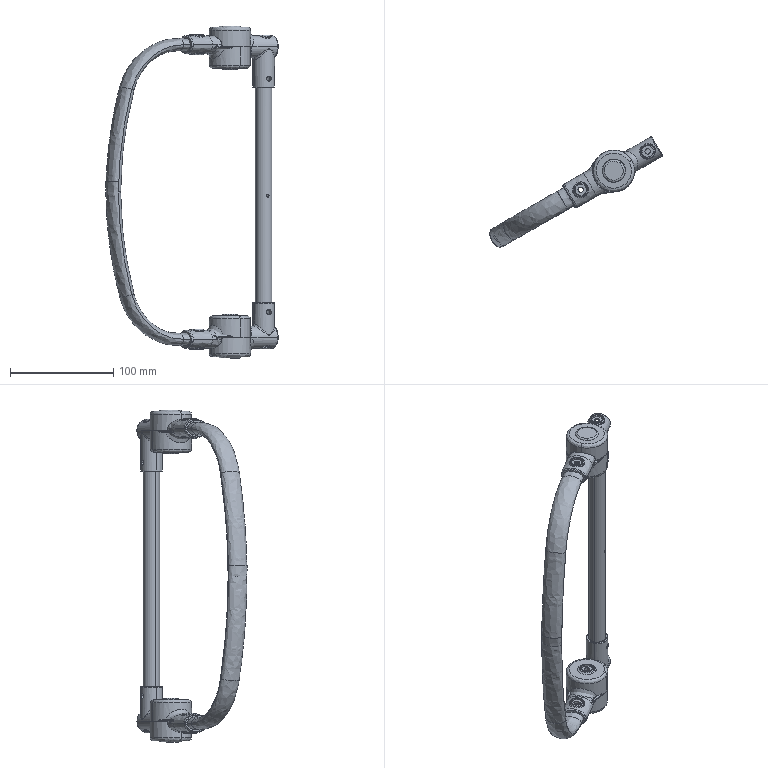Part | SolidWorks | 10 solids | 1235 faces | box 166.776 x 106.592 x 321.08 mm | volume 136620 mm3 | spline 635 | cylinder 345 | plane 230 | cone 14 | torus 11 | commonest cylinder face diameters 1.003 x58 5.2 x36 1 x30 34.6 x26 11 x16 14 x16